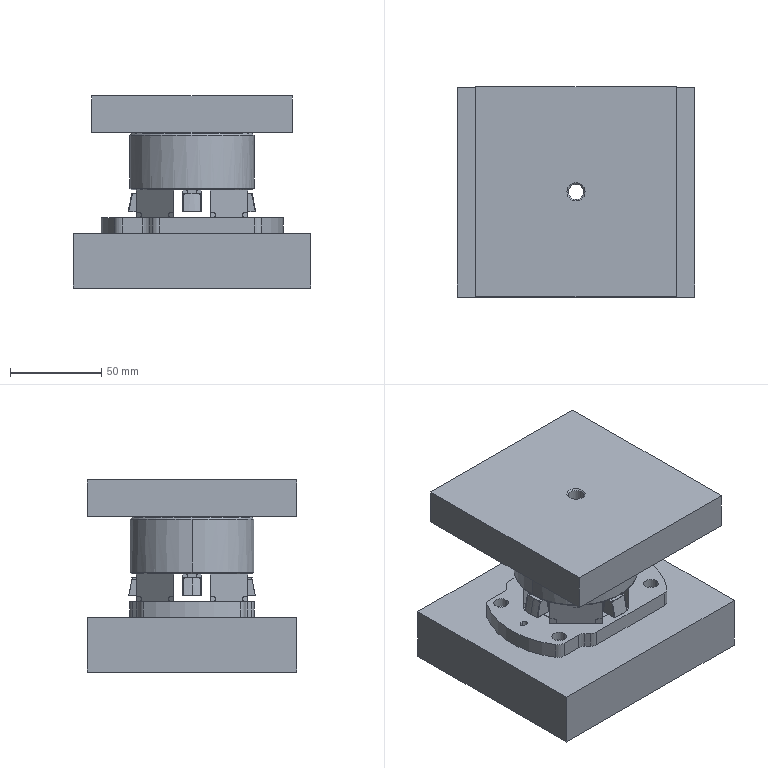NC program | NX | posted with a generic post | part box 130 x 115 x 105.2 mm
Lines 4072 to 4507 of 4507:
(138 , TOOL : ER25-D1.5-23_G)
N8040 T17 M6
N8042 G54
N8044 G17 G0 G90 X-14.075 Y-0.074 S5000 M3
N8046 G43 Z85. H17
N8048 G94 G1 Z32.5 F4500.
N8050 G41 X-14.025 Y-0.075 F300. D17
N8052 X-13.983 Y-0.074
N8054 X-13.951 Y-0.043
N8056 X-13.95 Y0.
N8058 Y5.05
N8060 Y5.25 F275.
N8062 Y5.45 F250.
N8064 Y5.65 F225.
N8066 Y5.85 F200.
N8068 Y6.05 F175.
N8070 Y6.25 F150.
N8072 X-14.45 F300.
N8074 Y6.05 F150.
N8076 Y5.85 F200.
N8078 Y5.65 F250.
N8080 Y-5.05 F300.
N8082 Y-5.25 F275.
N8084 Y-5.45 F250.
N8086 Y-5.65 F225.
N8088 Y-5.85 F200.
N8090 Y-6.05 F175.
N8092 Y-6.25 F150.
N8094 X-13.95 F300.
N8096 Y-6.05 F150.
N8098 Y-5.85 F200.
N8100 Y-5.65 F250.
N8102 Y0. F300.
N8104 Y0.5
N8106 X-13.951 Y0.543
N8108 X-13.983 Y0.574
N8110 X-14.025 Y0.575
N8112 G40
N8114 X-14.075 Y0.574
N8116 Y-0.074 Z30.5 F6000.
N8118 G41 X-14.025 Y-0.075 F300.
N8120 X-13.983 Y-0.074
N8122 X-13.951 Y-0.043
N8124 X-13.95 Y0.
N8126 Y5.05
N8128 Y5.25 F275.
N8130 Y5.45 F250.
N8132 Y5.65 F225.
N8134 Y5.85 F200.
N8136 Y6.05 F175.
N8138 Y6.25 F150.
N8140 X-14.45 F300.
N8142 Y6.05 F150.
N8144 Y5.85 F200.
N8146 Y5.65 F250.
N8148 Y-5.05 F300.
N8150 Y-5.25 F275.
N8152 Y-5.45 F250.
N8154 Y-5.65 F225.
N8156 Y-5.85 F200.
N8158 Y-6.05 F175.
N8160 Y-6.25 F150.
N8162 X-13.95 F300.
N8164 Y-6.05 F150.
N8166 Y-5.85 F200.
N8168 Y-5.65 F250.
N8170 Y0. F300.
N8172 Y0.5
N8174 X-13.951 Y0.543
N8176 X-13.983 Y0.574
N8178 X-14.025 Y0.575
N8180 G40
N8182 X-14.075 Y0.574
N8184 Y-0.074 Z29.55 F6000.
N8186 G41 X-14.025 Y-0.075 F300.
N8188 X-13.983 Y-0.074
N8190 X-13.951 Y-0.043
N8192 X-13.95 Y0.
N8194 Y5.05
N8196 Y5.25 F275.
N8198 Y5.45 F250.
N8200 Y5.65 F225.
N8202 Y5.85 F200.
N8204 Y6.05 F175.
N8206 Y6.25 F150.
N8208 X-14.45 F300.
N8210 Y6.05 F150.
N8212 Y5.85 F200.
N8214 Y5.65 F250.
N8216 Y-5.05 F300.
N8218 Y-5.25 F275.
N8220 Y-5.45 F250.
N8222 Y-5.65 F225.
N8224 Y-5.85 F200.
N8226 Y-6.05 F175.
N8228 Y-6.25 F150.
N8230 X-13.95 F300.
N8232 Y-6.05 F150.
N8234 Y-5.85 F200.
N8236 Y-5.65 F250.
N8238 Y0. F300.
N8240 Y0.5
N8242 X-13.951 Y0.543
N8244 X-13.983 Y0.574
N8246 X-14.025 Y0.575
N8248 G40
N8250 X-14.075 Y0.574
N8252 G0 Z85.
(PLANAR_MILL_1_5_COPY_4_COPY_COPY , TOOL : ER25-D1.5-23_G)
N8254 G18 X-14.125 Z-0.073
N8256 Y-85.
N8258 G1 Y-32.5 F4500.
N8260 G41 X-14.025 Z-0.075 F300.
N8262 X-13.988 Z-0.065
N8264 X-13.96 Z-0.038
N8266 X-13.95 Z0.
N8268 Z5.05
N8270 Z5.25 F275.
N8272 Z5.45 F250.
N8274 Z5.65 F225.
N8276 Z5.85 F200.
N8278 Z6.05 F175.
N8280 Z6.25 F150.
N8282 X-14.45 F300.
N8284 Z6.05 F150.
N8286 Z5.85 F200.
N8288 Z5.65 F250.
N8290 Z-5.05 F300.
N8292 Z-5.25 F275.
N8294 Z-5.45 F250.
N8296 Z-5.65 F225.
N8298 Z-5.85 F200.
N8300 Z-6.05 F175.
N8302 Z-6.25 F150.
N8304 X-13.95 F300.
N8306 Z-6.05 F150.
N8308 Z-5.85 F200.
N8310 Z-5.65 F250.
N8312 Z0. F300.
N8314 Z0.5
N8316 X-13.951 Z0.543
N8318 X-13.983 Z0.574
N8320 X-14.025 Z0.575
N8322 G40
N8324 X-14.125 Z0.573
N8326 Y-30.5 Z-0.073 F6000.
N8328 G41 X-14.025 Z-0.075 F300.
N8330 X-13.988 Z-0.065
N8332 X-13.96 Z-0.038
N8334 X-13.95 Z0.
N8336 Z5.05
N8338 Z5.25 F275.
N8340 Z5.45 F250.
N8342 Z5.65 F225.
N8344 Z5.85 F200.
N8346 Z6.05 F175.
N8348 Z6.25 F150.
N8350 X-14.45 F300.
N8352 Z6.05 F150.
N8354 Z5.85 F200.
N8356 Z5.65 F250.
N8358 Z-5.05 F300.
N8360 Z-5.25 F275.
N8362 Z-5.45 F250.
N8364 Z-5.65 F225.
N8366 Z-5.85 F200.
N8368 Z-6.05 F175.
N8370 Z-6.25 F150.
N8372 X-13.95 F300.
N8374 Z-6.05 F150.
N8376 Z-5.85 F200.
N8378 Z-5.65 F250.
N8380 Z0. F300.
N8382 Z0.5
N8384 X-13.951 Z0.543
N8386 X-13.983 Z0.574
N8388 X-14.025 Z0.575
N8390 G40
N8392 X-14.125 Z0.573
N8394 Y-29.55 Z-0.073 F6000.
N8396 G41 X-14.025 Z-0.075 F300.
N8398 X-13.988 Z-0.065
N8400 X-13.96 Z-0.038
N8402 X-13.95 Z0.
N8404 Z5.05
N8406 Z5.25 F275.
N8408 Z5.45 F250.
N8410 Z5.65 F225.
N8412 Z5.85 F200.
N8414 Z6.05 F175.
N8416 Z6.25 F150.
N8418 X-14.45 F300.
N8420 Z6.05 F150.
N8422 Z5.85 F200.
N8424 Z5.65 F250.
N8426 Z-5.05 F300.
N8428 Z-5.25 F275.
N8430 Z-5.45 F250.
N8432 Z-5.65 F225.
N8434 Z-5.85 F200.
N8436 Z-6.05 F175.
N8438 Z-6.25 F150.
N8440 X-13.95 F300.
N8442 Z-6.05 F150.
N8444 Z-5.85 F200.
N8446 Z-5.65 F250.
N8448 Z0. F300.
N8450 Z0.5
N8452 X-13.951 Z0.543
N8454 X-13.983 Z0.574
N8456 X-14.025 Z0.575
N8458 G40
N8460 X-14.125 Z0.573
N8462 G0 Y-85.
(PLANAR_MILL_1_5_COPY_4_COPY_COPY_1 , TOOL : ER25-D1.5-23_G)
N8464 G17 X-14.125 Y0.073
N8466 Z-85.
N8468 G1 Z-32.5 F4500.
N8470 G41 X-14.025 Y0.075 F300.
N8472 X-13.983 Y0.074
N8474 X-13.951 Y0.043
N8476 X-13.95 Y0.
N8478 Y-5.05
N8480 Y-5.25 F275.
N8482 Y-5.45 F250.
N8484 Y-5.65 F225.
N8486 Y-5.85 F200.
N8488 Y-6.05 F175.
N8490 Y-6.25 F150.
N8492 X-14.45 F300.
N8494 Y-6.05 F150.
N8496 Y-5.85 F200.
N8498 Y-5.65 F250.
N8500 Y5.05 F300.
N8502 Y5.25 F275.
N8504 Y5.45 F250.
N8506 Y5.65 F225.
N8508 Y5.85 F200.
N8510 Y6.05 F175.
N8512 Y6.25 F150.
N8514 X-13.95 F300.
N8516 Y6.05 F150.
N8518 Y5.85 F200.
N8520 Y5.65 F250.
N8522 Y0. F300.
N8524 Y-0.5
N8526 X-13.951 Y-0.543
N8528 X-13.983 Y-0.574
N8530 X-14.025 Y-0.575
N8532 G40
N8534 X-14.125 Y-0.573
N8536 Y0.073 Z-30.5 F6000.
N8538 G41 X-14.025 Y0.075 F300.
N8540 X-13.983 Y0.074
N8542 X-13.951 Y0.043
N8544 X-13.95 Y0.
N8546 Y-5.05
N8548 Y-5.25 F275.
N8550 Y-5.45 F250.
N8552 Y-5.65 F225.
N8554 Y-5.85 F200.
N8556 Y-6.05 F175.
N8558 Y-6.25 F150.
N8560 X-14.45 F300.
N8562 Y-6.05 F150.
N8564 Y-5.85 F200.
N8566 Y-5.65 F250.
N8568 Y5.05 F300.
N8570 Y5.25 F275.
N8572 Y5.45 F250.
N8574 Y5.65 F225.
N8576 Y5.85 F200.
N8578 Y6.05 F175.
N8580 Y6.25 F150.
N8582 X-13.95 F300.
N8584 Y6.05 F150.
N8586 Y5.85 F200.
N8588 Y5.65 F250.
N8590 Y0. F300.
N8592 Y-0.5
N8594 X-13.951 Y-0.543
N8596 X-13.983 Y-0.574
N8598 X-14.025 Y-0.575
N8600 G40
N8602 X-14.125 Y-0.573
N8604 Y0.073 Z-29.55 F6000.
N8606 G41 X-14.025 Y0.075 F300.
N8608 X-13.983 Y0.074
N8610 X-13.951 Y0.043
N8612 X-13.95 Y0.
N8614 Y-5.05
N8616 Y-5.25 F275.
N8618 Y-5.45 F250.
N8620 Y-5.65 F225.
N8622 Y-5.85 F200.
N8624 Y-6.05 F175.
N8626 Y-6.25 F150.
N8628 X-14.45 F300.
N8630 Y-6.05 F150.
N8632 Y-5.85 F200.
N8634 Y-5.65 F250.
N8636 Y5.05 F300.
N8638 Y5.25 F275.
N8640 Y5.45 F250.
N8642 Y5.65 F225.
N8644 Y5.85 F200.
N8646 Y6.05 F175.
N8648 Y6.25 F150.
N8650 X-13.95 F300.
N8652 Y6.05 F150.
N8654 Y5.85 F200.
N8656 Y5.65 F250.
N8658 Y0. F300.
N8660 Y-0.5
N8662 X-13.951 Y-0.543
N8664 X-13.983 Y-0.574
N8666 X-14.025 Y-0.575
N8668 G40
N8670 X-14.125 Y-0.573
N8672 G0 Z-85.
(PLANAR_MILL_1_5_COPY_4_COPY_COPY_2 , TOOL : ER25-D1.5-23_G)
N8674 G18 Y85.
N8676 X-14.125 Z0.073
N8678 G1 Y32.5 F4500.
N8680 G41 X-14.025 Z0.075 F300.
N8682 X-13.988 Z0.065
N8684 X-13.96 Z0.038
N8686 X-13.95 Z0.
N8688 Z-5.05
N8690 Z-5.25 F275.
N8692 Z-5.45 F250.
N8694 Z-5.65 F225.
N8696 Z-5.85 F200.
N8698 Z-6.05 F175.
N8700 Z-6.25 F150.
N8702 X-14.45 F300.
N8704 Z-6.05 F150.
N8706 Z-5.85 F200.
N8708 Z-5.65 F250.
N8710 Z5.05 F300.
N8712 Z5.25 F275.
N8714 Z5.45 F250.
N8716 Z5.65 F225.
N8718 Z5.85 F200.
N8720 Z6.05 F175.
N8722 Z6.25 F150.
N8724 X-13.95 F300.
N8726 Z6.05 F150.
N8728 Z5.85 F200.
N8730 Z5.65 F250.
N8732 Z0. F300.
N8734 Z-0.5
N8736 X-13.951 Z-0.543
N8738 X-13.983 Z-0.574
N8740 X-14.025 Z-0.575
N8742 G40
N8744 X-14.125 Z-0.573
N8746 Y30.5 Z0.073 F6000.
N8748 G41 X-14.025 Z0.075 F300.
N8750 X-13.988 Z0.065
N8752 X-13.96 Z0.038
N8754 X-13.95 Z0.
N8756 Z-5.05
N8758 Z-5.25 F275.
N8760 Z-5.45 F250.
N8762 Z-5.65 F225.
N8764 Z-5.85 F200.
N8766 Z-6.05 F175.
N8768 Z-6.25 F150.
N8770 X-14.45 F300.
N8772 Z-6.05 F150.
N8774 Z-5.85 F200.
N8776 Z-5.65 F250.
N8778 Z5.05 F300.
N8780 Z5.25 F275.
N8782 Z5.45 F250.
N8784 Z5.65 F225.
N8786 Z5.85 F200.
N8788 Z6.05 F175.
N8790 Z6.25 F150.
N8792 X-13.95 F300.
N8794 Z6.05 F150.
N8796 Z5.85 F200.
N8798 Z5.65 F250.
N8800 Z0. F300.
N8802 Z-0.5
N8804 X-13.951 Z-0.543
N8806 X-13.983 Z-0.574
N8808 X-14.025 Z-0.575
N8810 G40
N8812 X-14.125 Z-0.573
N8814 Y29.55 Z0.073 F6000.
N8816 G41 X-14.025 Z0.075 F300.
N8818 X-13.988 Z0.065
N8820 X-13.96 Z0.038
N8822 X-13.95 Z0.
N8824 Z-5.05
N8826 Z-5.25 F275.
N8828 Z-5.45 F250.
N8830 Z-5.65 F225.
N8832 Z-5.85 F200.
N8834 Z-6.05 F175.
N8836 Z-6.25 F150.
N8838 X-14.45 F300.
N8840 Z-6.05 F150.
N8842 Z-5.85 F200.
N8844 Z-5.65 F250.
N8846 Z5.05 F300.
N8848 Z5.25 F275.
N8850 Z5.45 F250.
N8852 Z5.65 F225.
N8854 Z5.85 F200.
N8856 Z6.05 F175.
N8858 Z6.25 F150.
N8860 X-13.95 F300.
N8862 Z6.05 F150.
N8864 Z5.85 F200.
N8866 Z5.65 F250.
N8868 Z0. F300.
N8870 Z-0.5
N8872 X-13.951 Z-0.543
N8874 X-13.983 Z-0.574
N8876 X-14.025 Z-0.575
N8878 G40
N8880 X-14.125 Z-0.573
N8882 G0 Y85.
N8884 M5
N8886 M2